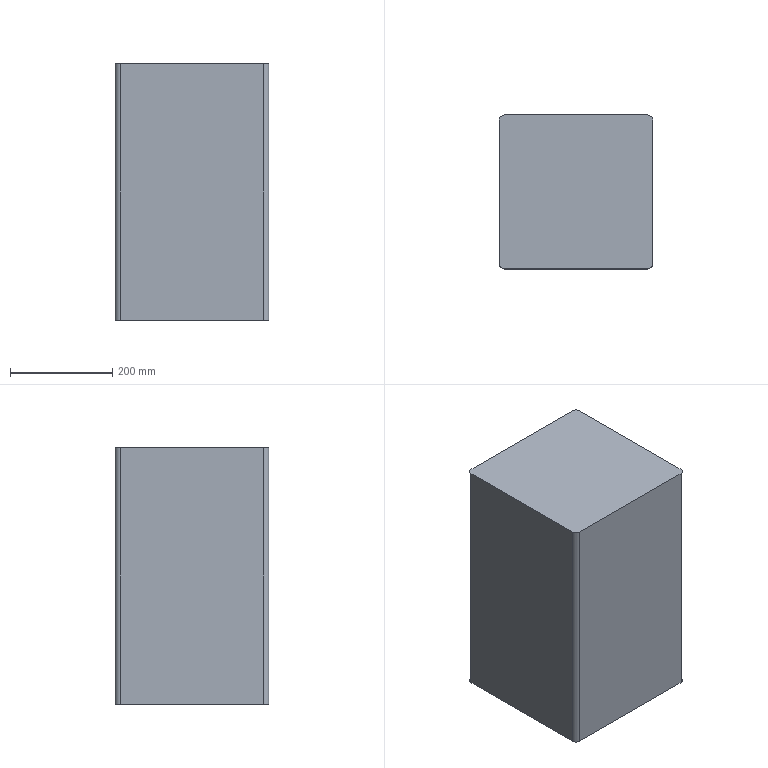Part | NX | features BREP 1 | 1 solid | 10 faces | box 300 x 300 x 500 mm | volume 44957080 mm3 | plane 6 | cylinder 4 | commonest cylinder face diameters 20 x4
STEP:
#1=CARTESIAN_POINT('',(150.,-140.,500.));
#2=VERTEX_POINT('',#1);
#3=CARTESIAN_POINT('',(150.,140.,500.));
#4=VERTEX_POINT('',#3);
#5=CARTESIAN_POINT('',(150.,150.,500.));
#6=DIRECTION('',(0.,1.,0.));
#7=VECTOR('',#6,1000.);
#8=LINE('',#5,#7);
#9=EDGE_CURVE('',#2,#4,#8,.T.);
#10=ORIENTED_EDGE('',*,*,#9,.F.);
#11=CARTESIAN_POINT('',(150.,-140.,0.));
#12=VERTEX_POINT('',#11);
#13=CARTESIAN_POINT('',(150.,-140.,500.));
#14=DIRECTION('',(0.,0.,-1.));
#15=VECTOR('',#14,1000.);
#16=LINE('',#13,#15);
#17=EDGE_CURVE('',#2,#12,#16,.T.);
#18=ORIENTED_EDGE('',*,*,#17,.T.);
#19=CARTESIAN_POINT('',(150.,140.,0.));
#20=VERTEX_POINT('',#19);
#21=CARTESIAN_POINT('',(150.,150.,0.));
#22=DIRECTION('',(0.,1.,0.));
#23=VECTOR('',#22,1000.);
#24=LINE('',#21,#23);
#25=EDGE_CURVE('',#12,#20,#24,.T.);
#26=ORIENTED_EDGE('',*,*,#25,.T.);
#27=CARTESIAN_POINT('',(150.,140.,500.));
#28=DIRECTION('',(0.,0.,1.));
#29=VECTOR('',#28,1000.);
#30=LINE('',#27,#29);
#31=EDGE_CURVE('',#20,#4,#30,.T.);
#32=ORIENTED_EDGE('',*,*,#31,.T.);
#33=EDGE_LOOP('',(#10,#18,#26,#32));
#34=FACE_BOUND('',#33,.T.);
#35=CARTESIAN_POINT('',(150.,150.,500.));
#36=DIRECTION('',(-1.,0.,0.));
#37=DIRECTION('',(0.,1.,0.));
#38=AXIS2_PLACEMENT_3D('',#35,#36,#37);
#39=PLANE('',#38);
#40=ADVANCED_FACE('',(#34),#39,.F.);
#41=CARTESIAN_POINT('',(140.,150.,500.));
#42=VERTEX_POINT('',#41);
#43=CARTESIAN_POINT('',(-140.,150.,500.));
#44=VERTEX_POINT('',#43);
#45=CARTESIAN_POINT('',(-150.,150.,500.));
#46=DIRECTION('',(-1.,0.,0.));
#47=VECTOR('',#46,1000.);
#48=LINE('',#45,#47);
#49=EDGE_CURVE('',#42,#44,#48,.T.);
#50=ORIENTED_EDGE('',*,*,#49,.F.);
#51=CARTESIAN_POINT('',(140.,150.,0.));
#52=VERTEX_POINT('',#51);
#53=CARTESIAN_POINT('',(140.,150.,500.));
#54=DIRECTION('',(0.,0.,-1.));
#55=VECTOR('',#54,1000.);
#56=LINE('',#53,#55);
#57=EDGE_CURVE('',#42,#52,#56,.T.);
#58=ORIENTED_EDGE('',*,*,#57,.T.);
#59=CARTESIAN_POINT('',(-140.,150.,0.));
#60=VERTEX_POINT('',#59);
#61=CARTESIAN_POINT('',(-150.,150.,0.));
#62=DIRECTION('',(-1.,0.,0.));
#63=VECTOR('',#62,1000.);
#64=LINE('',#61,#63);
#65=EDGE_CURVE('',#52,#60,#64,.T.);
#66=ORIENTED_EDGE('',*,*,#65,.T.);
#67=CARTESIAN_POINT('',(-140.,150.,500.));
#68=DIRECTION('',(0.,0.,1.));
#69=VECTOR('',#68,1000.);
#70=LINE('',#67,#69);
#71=EDGE_CURVE('',#60,#44,#70,.T.);
#72=ORIENTED_EDGE('',*,*,#71,.T.);
#73=EDGE_LOOP('',(#50,#58,#66,#72));
#74=FACE_BOUND('',#73,.T.);
#75=CARTESIAN_POINT('',(-150.,150.,500.));
#76=DIRECTION('',(0.,-1.,0.));
#77=DIRECTION('',(0.,0.,-1.));
#78=AXIS2_PLACEMENT_3D('',#75,#76,#77);
#79=PLANE('',#78);
#80=ADVANCED_FACE('',(#74),#79,.F.);
#81=CARTESIAN_POINT('',(-150.,140.,0.));
#82=VERTEX_POINT('',#81);
#83=CARTESIAN_POINT('',(-150.,-140.,0.));
#84=VERTEX_POINT('',#83);
#85=CARTESIAN_POINT('',(-150.,150.,0.));
#86=DIRECTION('',(0.,-1.,0.));
#87=VECTOR('',#86,1000.);
#88=LINE('',#85,#87);
#89=EDGE_CURVE('',#82,#84,#88,.T.);
#90=ORIENTED_EDGE('',*,*,#89,.T.);
#91=CARTESIAN_POINT('',(-150.,-140.,500.));
#92=VERTEX_POINT('',#91);
#93=CARTESIAN_POINT('',(-150.,-140.,500.));
#94=DIRECTION('',(0.,0.,1.));
#95=VECTOR('',#94,1000.);
#96=LINE('',#93,#95);
#97=EDGE_CURVE('',#84,#92,#96,.T.);
#98=ORIENTED_EDGE('',*,*,#97,.T.);
#99=CARTESIAN_POINT('',(-150.,140.,500.));
#100=VERTEX_POINT('',#99);
#101=CARTESIAN_POINT('',(-150.,150.,500.));
#102=DIRECTION('',(0.,-1.,0.));
#103=VECTOR('',#102,1000.);
#104=LINE('',#101,#103);
#105=EDGE_CURVE('',#100,#92,#104,.T.);
#106=ORIENTED_EDGE('',*,*,#105,.F.);
#107=CARTESIAN_POINT('',(-150.,140.,500.));
#108=DIRECTION('',(0.,0.,-1.));
#109=VECTOR('',#108,1000.);
#110=LINE('',#107,#109);
#111=EDGE_CURVE('',#100,#82,#110,.T.);
#112=ORIENTED_EDGE('',*,*,#111,.T.);
#113=EDGE_LOOP('',(#90,#98,#106,#112));
#114=FACE_BOUND('',#113,.T.);
#115=CARTESIAN_POINT('',(-150.,150.,500.));
#116=DIRECTION('',(1.,0.,0.));
#117=DIRECTION('',(0.,1.,0.));
#118=AXIS2_PLACEMENT_3D('',#115,#116,#117);
#119=PLANE('',#118);
#120=ADVANCED_FACE('',(#114),#119,.F.);
#121=CARTESIAN_POINT('',(-140.,-150.,500.));
#122=VERTEX_POINT('',#121);
#123=CARTESIAN_POINT('',(140.,-150.,500.));
#124=VERTEX_POINT('',#123);
#125=CARTESIAN_POINT('',(-150.,-150.,500.));
#126=DIRECTION('',(1.,0.,0.));
#127=VECTOR('',#126,1000.);
#128=LINE('',#125,#127);
#129=EDGE_CURVE('',#122,#124,#128,.T.);
#130=ORIENTED_EDGE('',*,*,#129,.F.);
#131=CARTESIAN_POINT('',(-140.,-150.,0.));
#132=VERTEX_POINT('',#131);
#133=CARTESIAN_POINT('',(-140.,-150.,500.));
#134=DIRECTION('',(0.,0.,-1.));
#135=VECTOR('',#134,1000.);
#136=LINE('',#133,#135);
#137=EDGE_CURVE('',#122,#132,#136,.T.);
#138=ORIENTED_EDGE('',*,*,#137,.T.);
#139=CARTESIAN_POINT('',(140.,-150.,0.));
#140=VERTEX_POINT('',#139);
#141=CARTESIAN_POINT('',(-150.,-150.,0.));
#142=DIRECTION('',(1.,0.,0.));
#143=VECTOR('',#142,1000.);
#144=LINE('',#141,#143);
#145=EDGE_CURVE('',#132,#140,#144,.T.);
#146=ORIENTED_EDGE('',*,*,#145,.T.);
#147=CARTESIAN_POINT('',(140.,-150.,500.));
#148=DIRECTION('',(0.,0.,1.));
#149=VECTOR('',#148,1000.);
#150=LINE('',#147,#149);
#151=EDGE_CURVE('',#140,#124,#150,.T.);
#152=ORIENTED_EDGE('',*,*,#151,.T.);
#153=EDGE_LOOP('',(#130,#138,#146,#152));
#154=FACE_BOUND('',#153,.T.);
#155=CARTESIAN_POINT('',(-150.,-150.,500.));
#156=DIRECTION('',(0.,1.,0.));
#157=DIRECTION('',(1.,0.,0.));
#158=AXIS2_PLACEMENT_3D('',#155,#156,#157);
#159=PLANE('',#158);
#160=ADVANCED_FACE('',(#154),#159,.F.);
#161=ORIENTED_EDGE('',*,*,#105,.T.);
#162=CARTESIAN_POINT('',(-140.,-140.,500.));
#163=DIRECTION('',(0.,0.,1.));
#164=DIRECTION('',(1.,0.,0.));
#165=AXIS2_PLACEMENT_3D('',#162,#163,#164);
#166=CIRCLE('',#165,10.);
#167=EDGE_CURVE('',#92,#122,#166,.T.);
#168=ORIENTED_EDGE('',*,*,#167,.T.);
#169=ORIENTED_EDGE('',*,*,#129,.T.);
#170=CARTESIAN_POINT('',(140.,-140.,500.));
#171=DIRECTION('',(0.,0.,1.));
#172=DIRECTION('',(1.,0.,0.));
#173=AXIS2_PLACEMENT_3D('',#170,#171,#172);
#174=CIRCLE('',#173,10.);
#175=EDGE_CURVE('',#124,#2,#174,.T.);
#176=ORIENTED_EDGE('',*,*,#175,.T.);
#177=ORIENTED_EDGE('',*,*,#9,.T.);
#178=CARTESIAN_POINT('',(140.,140.,500.));
#179=DIRECTION('',(0.,0.,1.));
#180=DIRECTION('',(1.,0.,0.));
#181=AXIS2_PLACEMENT_3D('',#178,#179,#180);
#182=CIRCLE('',#181,10.);
#183=EDGE_CURVE('',#4,#42,#182,.T.);
#184=ORIENTED_EDGE('',*,*,#183,.T.);
#185=ORIENTED_EDGE('',*,*,#49,.T.);
#186=CARTESIAN_POINT('',(-140.,140.,500.));
#187=DIRECTION('',(0.,0.,1.));
#188=DIRECTION('',(1.,0.,0.));
#189=AXIS2_PLACEMENT_3D('',#186,#187,#188);
#190=CIRCLE('',#189,10.);
#191=EDGE_CURVE('',#44,#100,#190,.T.);
#192=ORIENTED_EDGE('',*,*,#191,.T.);
#193=EDGE_LOOP('',(#161,#168,#169,#176,#177,#184,#185,#192));
#194=FACE_BOUND('',#193,.T.);
#195=CARTESIAN_POINT('',(0.,0.,500.));
#196=DIRECTION('',(0.,0.,1.));
#197=DIRECTION('',(1.,0.,0.));
#198=AXIS2_PLACEMENT_3D('',#195,#196,#197);
#199=PLANE('',#198);
#200=ADVANCED_FACE('',(#194),#199,.T.);
#201=ORIENTED_EDGE('',*,*,#145,.F.);
#202=CARTESIAN_POINT('',(-140.,-140.,0.));
#203=DIRECTION('',(0.,0.,-1.));
#204=DIRECTION('',(1.,0.,0.));
#205=AXIS2_PLACEMENT_3D('',#202,#203,#204);
#206=CIRCLE('',#205,10.);
#207=EDGE_CURVE('',#132,#84,#206,.T.);
#208=ORIENTED_EDGE('',*,*,#207,.T.);
#209=ORIENTED_EDGE('',*,*,#89,.F.);
#210=CARTESIAN_POINT('',(-140.,140.,0.));
#211=DIRECTION('',(0.,0.,-1.));
#212=DIRECTION('',(1.,0.,0.));
#213=AXIS2_PLACEMENT_3D('',#210,#211,#212);
#214=CIRCLE('',#213,10.);
#215=EDGE_CURVE('',#82,#60,#214,.T.);
#216=ORIENTED_EDGE('',*,*,#215,.T.);
#217=ORIENTED_EDGE('',*,*,#65,.F.);
#218=CARTESIAN_POINT('',(140.,140.,0.));
#219=DIRECTION('',(0.,0.,-1.));
#220=DIRECTION('',(1.,0.,0.));
#221=AXIS2_PLACEMENT_3D('',#218,#219,#220);
#222=CIRCLE('',#221,10.);
#223=EDGE_CURVE('',#52,#20,#222,.T.);
#224=ORIENTED_EDGE('',*,*,#223,.T.);
#225=ORIENTED_EDGE('',*,*,#25,.F.);
#226=CARTESIAN_POINT('',(140.,-140.,0.));
#227=DIRECTION('',(0.,0.,-1.));
#228=DIRECTION('',(1.,0.,0.));
#229=AXIS2_PLACEMENT_3D('',#226,#227,#228);
#230=CIRCLE('',#229,10.);
#231=EDGE_CURVE('',#12,#140,#230,.T.);
#232=ORIENTED_EDGE('',*,*,#231,.T.);
#233=EDGE_LOOP('',(#201,#208,#209,#216,#217,#224,#225,#232));
#234=FACE_BOUND('',#233,.T.);
#235=CARTESIAN_POINT('',(0.,0.,0.));
#236=DIRECTION('',(0.,0.,1.));
#237=DIRECTION('',(1.,0.,0.));
#238=AXIS2_PLACEMENT_3D('',#235,#236,#237);
#239=PLANE('',#238);
#240=ADVANCED_FACE('',(#234),#239,.F.);
#241=ORIENTED_EDGE('',*,*,#167,.F.);
#242=ORIENTED_EDGE('',*,*,#97,.F.);
#243=ORIENTED_EDGE('',*,*,#207,.F.);
#244=ORIENTED_EDGE('',*,*,#137,.F.);
#245=EDGE_LOOP('',(#241,#242,#243,#244));
#246=FACE_BOUND('',#245,.T.);
#247=CARTESIAN_POINT('',(-140.,-140.,500.));
#248=DIRECTION('',(0.,0.,-1.));
#249=DIRECTION('',(-1.,0.,0.));
#250=AXIS2_PLACEMENT_3D('',#247,#248,#249);
#251=CYLINDRICAL_SURFACE('',#250,10.);
#252=ADVANCED_FACE('',(#246),#251,.T.);
#253=ORIENTED_EDGE('',*,*,#175,.F.);
#254=ORIENTED_EDGE('',*,*,#151,.F.);
#255=ORIENTED_EDGE('',*,*,#231,.F.);
#256=ORIENTED_EDGE('',*,*,#17,.F.);
#257=EDGE_LOOP('',(#253,#254,#255,#256));
#258=FACE_BOUND('',#257,.T.);
#259=CARTESIAN_POINT('',(140.,-140.,500.));
#260=DIRECTION('',(0.,0.,-1.));
#261=DIRECTION('',(-1.,0.,0.));
#262=AXIS2_PLACEMENT_3D('',#259,#260,#261);
#263=CYLINDRICAL_SURFACE('',#262,10.);
#264=ADVANCED_FACE('',(#258),#263,.T.);
#265=ORIENTED_EDGE('',*,*,#183,.F.);
#266=ORIENTED_EDGE('',*,*,#31,.F.);
#267=ORIENTED_EDGE('',*,*,#223,.F.);
#268=ORIENTED_EDGE('',*,*,#57,.F.);
#269=EDGE_LOOP('',(#265,#266,#267,#268));
#270=FACE_BOUND('',#269,.T.);
#271=CARTESIAN_POINT('',(140.,140.,500.));
#272=DIRECTION('',(0.,0.,-1.));
#273=DIRECTION('',(-1.,0.,0.));
#274=AXIS2_PLACEMENT_3D('',#271,#272,#273);
#275=CYLINDRICAL_SURFACE('',#274,10.);
#276=ADVANCED_FACE('',(#270),#275,.T.);
#277=ORIENTED_EDGE('',*,*,#191,.F.);
#278=ORIENTED_EDGE('',*,*,#71,.F.);
#279=ORIENTED_EDGE('',*,*,#215,.F.);
#280=ORIENTED_EDGE('',*,*,#111,.F.);
#281=EDGE_LOOP('',(#277,#278,#279,#280));
#282=FACE_BOUND('',#281,.T.);
#283=CARTESIAN_POINT('',(-140.,140.,500.));
#284=DIRECTION('',(0.,0.,-1.));
#285=DIRECTION('',(-1.,0.,0.));
#286=AXIS2_PLACEMENT_3D('',#283,#284,#285);
#287=CYLINDRICAL_SURFACE('',#286,10.);
#288=ADVANCED_FACE('',(#282),#287,.T.);
#289=CLOSED_SHELL('',(#40,#80,#120,#160,#200,#240,#252,#264,#276,#288));
#290=MANIFOLD_SOLID_BREP('',#289);
#291=(LENGTH_UNIT()NAMED_UNIT(*)SI_UNIT(.MILLI.,.METRE.));
#292=UNCERTAINTY_MEASURE_WITH_UNIT(LENGTH_MEASURE(0.00001),#291,'','');
#293=(NAMED_UNIT(*)PLANE_ANGLE_UNIT()SI_UNIT($,.RADIAN.));
#294=(NAMED_UNIT(*)SI_UNIT($,.STERADIAN.)SOLID_ANGLE_UNIT());
#295=(GEOMETRIC_REPRESENTATION_CONTEXT(3)GLOBAL_UNCERTAINTY_ASSIGNED_CONTEXT((#292))GLOBAL_UNIT_ASSIGNED_CONTEXT((#291,#293,#294))REPRESENTATION_CONTEXT('',''));
#296=ADVANCED_BREP_SHAPE_REPRESENTATION('',(#290),#295);